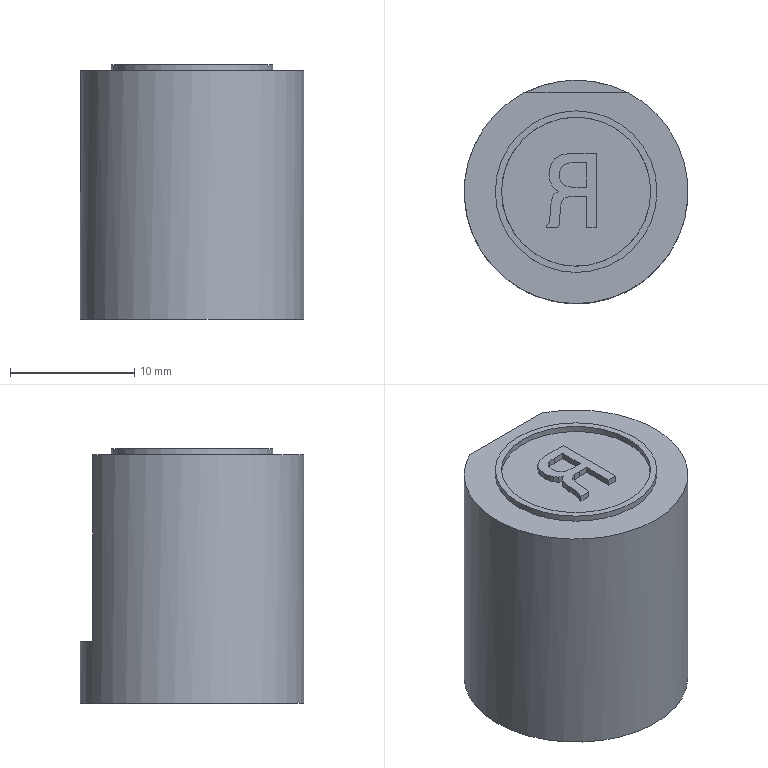Part | STEP file | lll_id4346_x_t | 1 solid | 50 faces | box 18 x 18 x 20.5 mm | volume 5022 mm3 | plane 47 | cylinder 3 | commonest cylinder face diameters 12 x1 13 x1 18 x1
STEP:
#1=CARTESIAN_POINT('',(396.,100.,0.));
#2=VERTEX_POINT('',#1);
#3=CARTESIAN_POINT('',(389.5,100.,0.));
#4=DIRECTION('',(0.,0.,-1.));
#5=DIRECTION('',(1.,0.,0.));
#6=AXIS2_PLACEMENT_3D('',#3,#4,#5);
#7=CIRCLE('',#6,6.5);
#8=EDGE_CURVE('',#2,#2,#7,.T.);
#9=ORIENTED_EDGE('',*,*,#8,.T.);
#10=EDGE_LOOP('',(#9));
#11=FACE_BOUND('',#10,.T.);
#12=CARTESIAN_POINT('',(393.623,108.,0.));
#13=VERTEX_POINT('',#12);
#14=CARTESIAN_POINT('',(385.377,108.,0.));
#15=VERTEX_POINT('',#14);
#16=CARTESIAN_POINT('',(389.5,108.,0.));
#17=DIRECTION('',(-1.,0.,0.));
#18=VECTOR('',#17,1.);
#19=LINE('',#16,#18);
#20=EDGE_CURVE('',#13,#15,#19,.T.);
#21=ORIENTED_EDGE('',*,*,#20,.T.);
#22=CARTESIAN_POINT('',(389.5,100.,0.));
#23=DIRECTION('',(0.,0.,-1.));
#24=DIRECTION('',(-1.,0.,0.));
#25=AXIS2_PLACEMENT_3D('',#22,#23,#24);
#26=CIRCLE('',#25,9.);
#27=EDGE_CURVE('',#13,#15,#26,.T.);
#28=ORIENTED_EDGE('',*,*,#27,.F.);
#29=EDGE_LOOP('',(#21,#28));
#30=FACE_BOUND('',#29,.T.);
#31=CARTESIAN_POINT('',(389.5,100.,0.));
#32=DIRECTION('',(0.,0.,1.));
#33=DIRECTION('',(1.,0.,0.));
#34=AXIS2_PLACEMENT_3D('',#31,#32,#33);
#35=PLANE('',#34);
#36=ADVANCED_FACE('',(#11,#30),#35,.T.);
#37=CARTESIAN_POINT('',(395.5,100.,0.));
#38=VERTEX_POINT('',#37);
#39=CARTESIAN_POINT('',(389.5,100.,0.));
#40=DIRECTION('',(0.,0.,1.));
#41=DIRECTION('',(1.,0.,0.));
#42=AXIS2_PLACEMENT_3D('',#39,#40,#41);
#43=CIRCLE('',#42,6.);
#44=EDGE_CURVE('',#38,#38,#43,.T.);
#45=ORIENTED_EDGE('',*,*,#44,.T.);
#46=EDGE_LOOP('',(#45));
#47=FACE_BOUND('',#46,.T.);
#48=CARTESIAN_POINT('',(388.133,97.386,0.));
#49=VERTEX_POINT('',#48);
#50=CARTESIAN_POINT('',(388.185,97.896,0.));
#51=VERTEX_POINT('',#50);
#52=CARTESIAN_POINT('',(388.133,97.386,0.));
#53=DIRECTION('',(0.1012,0.9949,0.));
#54=VECTOR('',#53,1.);
#55=LINE('',#52,#54);
#56=EDGE_CURVE('',#49,#51,#55,.T.);
#57=ORIENTED_EDGE('',*,*,#56,.F.);
#58=CARTESIAN_POINT('',(388.029,97.083,0.));
#59=VERTEX_POINT('',#58);
#60=CARTESIAN_POINT('',(388.029,97.083,0.));
#61=DIRECTION('',(-0.3242,-0.946,0.));
#62=VECTOR('',#61,1.);
#63=LINE('',#60,#62);
#64=EDGE_CURVE('',#49,#59,#63,.T.);
#65=ORIENTED_EDGE('',*,*,#64,.T.);
#66=CARTESIAN_POINT('',(387.121,97.083,0.));
#67=VERTEX_POINT('',#66);
#68=CARTESIAN_POINT('',(387.121,97.083,0.));
#69=DIRECTION('',(-1.,0.,0.));
#70=VECTOR('',#69,1.);
#71=LINE('',#68,#70);
#72=EDGE_CURVE('',#59,#67,#71,.T.);
#73=ORIENTED_EDGE('',*,*,#72,.T.);
#74=CARTESIAN_POINT('',(387.121,97.247,0.));
#75=VERTEX_POINT('',#74);
#76=CARTESIAN_POINT('',(387.121,97.247,0.));
#77=DIRECTION('',(0.,1.,0.));
#78=VECTOR('',#77,1.);
#79=LINE('',#76,#78);
#80=EDGE_CURVE('',#67,#75,#79,.T.);
#81=ORIENTED_EDGE('',*,*,#80,.T.);
#82=CARTESIAN_POINT('',(387.32,97.489,0.));
#83=VERTEX_POINT('',#82);
#84=CARTESIAN_POINT('',(387.32,97.489,0.));
#85=DIRECTION('',(0.6346,0.7728,0.));
#86=VECTOR('',#85,1.);
#87=LINE('',#84,#86);
#88=EDGE_CURVE('',#75,#83,#87,.T.);
#89=ORIENTED_EDGE('',*,*,#88,.T.);
#90=CARTESIAN_POINT('',(387.389,97.939,0.));
#91=VERTEX_POINT('',#90);
#92=CARTESIAN_POINT('',(387.389,97.939,0.));
#93=DIRECTION('',(0.1522,0.9884,0.));
#94=VECTOR('',#93,1.);
#95=LINE('',#92,#94);
#96=EDGE_CURVE('',#83,#91,#95,.T.);
#97=ORIENTED_EDGE('',*,*,#96,.T.);
#98=CARTESIAN_POINT('',(387.45,98.907,0.));
#99=VERTEX_POINT('',#98);
#100=CARTESIAN_POINT('',(387.45,98.907,0.));
#101=DIRECTION('',(-0.06234,-0.9981,0.));
#102=VECTOR('',#101,1.);
#103=LINE('',#100,#102);
#104=EDGE_CURVE('',#99,#91,#103,.T.);
#105=ORIENTED_EDGE('',*,*,#104,.F.);
#106=CARTESIAN_POINT('',(387.597,99.625,0.));
#107=VERTEX_POINT('',#106);
#108=CARTESIAN_POINT('',(387.597,99.625,0.));
#109=DIRECTION('',(-0.2007,-0.9797,0.));
#110=VECTOR('',#109,1.);
#111=LINE('',#108,#110);
#112=EDGE_CURVE('',#107,#99,#111,.T.);
#113=ORIENTED_EDGE('',*,*,#112,.F.);
#114=CARTESIAN_POINT('',(387.796,99.85,0.));
#115=VERTEX_POINT('',#114);
#116=CARTESIAN_POINT('',(387.796,99.85,0.));
#117=DIRECTION('',(0.6626,0.749,0.));
#118=VECTOR('',#117,1.);
#119=LINE('',#116,#118);
#120=EDGE_CURVE('',#107,#115,#119,.T.);
#121=ORIENTED_EDGE('',*,*,#120,.T.);
#122=CARTESIAN_POINT('',(388.107,100.014,0.));
#123=VERTEX_POINT('',#122);
#124=CARTESIAN_POINT('',(388.107,100.014,0.));
#125=DIRECTION('',(0.8844,0.4668,0.));
#126=VECTOR('',#125,1.);
#127=LINE('',#124,#126);
#128=EDGE_CURVE('',#115,#123,#127,.T.);
#129=ORIENTED_EDGE('',*,*,#128,.T.);
#130=CARTESIAN_POINT('',(387.761,100.23,0.));
#131=VERTEX_POINT('',#130);
#132=CARTESIAN_POINT('',(387.761,100.23,0.));
#133=DIRECTION('',(0.848,-0.53,0.));
#134=VECTOR('',#133,1.);
#135=LINE('',#132,#134);
#136=EDGE_CURVE('',#131,#123,#135,.T.);
#137=ORIENTED_EDGE('',*,*,#136,.F.);
#138=CARTESIAN_POINT('',(387.519,100.533,0.));
#139=VERTEX_POINT('',#138);
#140=CARTESIAN_POINT('',(387.519,100.533,0.));
#141=DIRECTION('',(-0.6248,0.7808,0.));
#142=VECTOR('',#141,1.);
#143=LINE('',#140,#142);
#144=EDGE_CURVE('',#131,#139,#143,.T.);
#145=ORIENTED_EDGE('',*,*,#144,.T.);
#146=CARTESIAN_POINT('',(387.363,100.913,0.));
#147=VERTEX_POINT('',#146);
#148=CARTESIAN_POINT('',(387.363,100.913,0.));
#149=DIRECTION('',(0.3785,-0.9256,0.));
#150=VECTOR('',#149,1.);
#151=LINE('',#148,#150);
#152=EDGE_CURVE('',#147,#139,#151,.T.);
#153=ORIENTED_EDGE('',*,*,#152,.F.);
#154=CARTESIAN_POINT('',(387.312,101.371,0.));
#155=VERTEX_POINT('',#154);
#156=CARTESIAN_POINT('',(387.312,101.371,0.));
#157=DIRECTION('',(-0.1125,0.9937,0.));
#158=VECTOR('',#157,1.);
#159=LINE('',#156,#158);
#160=EDGE_CURVE('',#147,#155,#159,.T.);
#161=ORIENTED_EDGE('',*,*,#160,.T.);
#162=CARTESIAN_POINT('',(387.433,102.098,0.));
#163=VERTEX_POINT('',#162);
#164=CARTESIAN_POINT('',(387.433,102.098,0.));
#165=DIRECTION('',(-0.1644,-0.9864,0.));
#166=VECTOR('',#165,1.);
#167=LINE('',#164,#166);
#168=EDGE_CURVE('',#163,#155,#167,.T.);
#169=ORIENTED_EDGE('',*,*,#168,.F.);
#170=CARTESIAN_POINT('',(387.778,102.642,0.));
#171=VERTEX_POINT('',#170);
#172=CARTESIAN_POINT('',(387.778,102.642,0.));
#173=DIRECTION('',(0.536,0.8442,0.));
#174=VECTOR('',#173,1.);
#175=LINE('',#172,#174);
#176=EDGE_CURVE('',#163,#171,#175,.T.);
#177=ORIENTED_EDGE('',*,*,#176,.T.);
#178=CARTESIAN_POINT('',(388.349,102.971,0.));
#179=VERTEX_POINT('',#178);
#180=CARTESIAN_POINT('',(388.349,102.971,0.));
#181=DIRECTION('',(0.8666,0.4989,0.));
#182=VECTOR('',#181,1.);
#183=LINE('',#180,#182);
#184=EDGE_CURVE('',#171,#179,#183,.T.);
#185=ORIENTED_EDGE('',*,*,#184,.T.);
#186=CARTESIAN_POINT('',(389.127,103.083,0.));
#187=VERTEX_POINT('',#186);
#188=CARTESIAN_POINT('',(389.127,103.083,0.));
#189=DIRECTION('',(0.9897,0.143,0.));
#190=VECTOR('',#189,1.);
#191=LINE('',#188,#190);
#192=EDGE_CURVE('',#179,#187,#191,.T.);
#193=ORIENTED_EDGE('',*,*,#192,.T.);
#194=CARTESIAN_POINT('',(391.133,103.083,0.));
#195=VERTEX_POINT('',#194);
#196=CARTESIAN_POINT('',(391.133,103.083,0.));
#197=DIRECTION('',(-1.,0.,0.));
#198=VECTOR('',#197,1.);
#199=LINE('',#196,#198);
#200=EDGE_CURVE('',#195,#187,#199,.T.);
#201=ORIENTED_EDGE('',*,*,#200,.F.);
#202=CARTESIAN_POINT('',(391.133,97.083,0.));
#203=VERTEX_POINT('',#202);
#204=CARTESIAN_POINT('',(391.133,97.083,0.));
#205=DIRECTION('',(0.,-1.,0.));
#206=VECTOR('',#205,1.);
#207=LINE('',#204,#206);
#208=EDGE_CURVE('',#195,#203,#207,.T.);
#209=ORIENTED_EDGE('',*,*,#208,.T.);
#210=CARTESIAN_POINT('',(390.329,97.083,0.));
#211=VERTEX_POINT('',#210);
#212=CARTESIAN_POINT('',(390.329,97.083,0.));
#213=DIRECTION('',(1.,0.,0.));
#214=VECTOR('',#213,1.);
#215=LINE('',#212,#214);
#216=EDGE_CURVE('',#211,#203,#215,.T.);
#217=ORIENTED_EDGE('',*,*,#216,.F.);
#218=CARTESIAN_POINT('',(390.329,99.616,0.));
#219=VERTEX_POINT('',#218);
#220=CARTESIAN_POINT('',(390.329,99.616,0.));
#221=DIRECTION('',(0.,-1.,0.));
#222=VECTOR('',#221,1.);
#223=LINE('',#220,#222);
#224=EDGE_CURVE('',#219,#211,#223,.T.);
#225=ORIENTED_EDGE('',*,*,#224,.F.);
#226=CARTESIAN_POINT('',(389.508,99.616,0.));
#227=VERTEX_POINT('',#226);
#228=CARTESIAN_POINT('',(389.508,99.616,0.));
#229=DIRECTION('',(-1.,0.,0.));
#230=VECTOR('',#229,1.);
#231=LINE('',#228,#230);
#232=EDGE_CURVE('',#219,#227,#231,.T.);
#233=ORIENTED_EDGE('',*,*,#232,.T.);
#234=CARTESIAN_POINT('',(388.902,99.59,0.));
#235=VERTEX_POINT('',#234);
#236=CARTESIAN_POINT('',(388.902,99.59,0.));
#237=DIRECTION('',(-0.9991,-0.04282,0.));
#238=VECTOR('',#237,1.);
#239=LINE('',#236,#238);
#240=EDGE_CURVE('',#227,#235,#239,.T.);
#241=ORIENTED_EDGE('',*,*,#240,.T.);
#242=CARTESIAN_POINT('',(388.522,99.469,0.));
#243=VERTEX_POINT('',#242);
#244=CARTESIAN_POINT('',(388.522,99.469,0.));
#245=DIRECTION('',(0.9529,0.3032,0.));
#246=VECTOR('',#245,1.);
#247=LINE('',#244,#246);
#248=EDGE_CURVE('',#243,#235,#247,.T.);
#249=ORIENTED_EDGE('',*,*,#248,.F.);
#250=CARTESIAN_POINT('',(388.314,99.184,0.));
#251=VERTEX_POINT('',#250);
#252=CARTESIAN_POINT('',(388.314,99.184,0.));
#253=DIRECTION('',(-0.5882,-0.8087,0.));
#254=VECTOR('',#253,1.);
#255=LINE('',#252,#254);
#256=EDGE_CURVE('',#243,#251,#255,.T.);
#257=ORIENTED_EDGE('',*,*,#256,.T.);
#258=CARTESIAN_POINT('',(388.228,98.674,0.));
#259=VERTEX_POINT('',#258);
#260=CARTESIAN_POINT('',(388.228,98.674,0.));
#261=DIRECTION('',(0.1671,0.9859,0.));
#262=VECTOR('',#261,1.);
#263=LINE('',#260,#262);
#264=EDGE_CURVE('',#259,#251,#263,.T.);
#265=ORIENTED_EDGE('',*,*,#264,.F.);
#266=CARTESIAN_POINT('',(388.185,97.896,0.));
#267=DIRECTION('',(-0.05553,-0.9985,0.));
#268=VECTOR('',#267,1.);
#269=LINE('',#266,#268);
#270=EDGE_CURVE('',#259,#51,#269,.T.);
#271=ORIENTED_EDGE('',*,*,#270,.T.);
#272=EDGE_LOOP('',(#57,#65,#73,#81,#89,#97,#105,#113,#121,#129,#137,#145,#153,#161,#169,#177,#185,#193,#201,#209,#217,#225,#233,#241,#249,#257,#265,#271));
#273=FACE_BOUND('',#272,.T.);
#274=CARTESIAN_POINT('',(389.5,100.,0.));
#275=DIRECTION('',(0.,0.,1.));
#276=DIRECTION('',(1.,0.,0.));
#277=AXIS2_PLACEMENT_3D('',#274,#275,#276);
#278=PLANE('',#277);
#279=ADVANCED_FACE('',(#47,#273),#278,.T.);
#280=ORIENTED_EDGE('',*,*,#8,.F.);
#281=EDGE_LOOP('',(#280));
#282=FACE_BOUND('',#281,.T.);
#283=CARTESIAN_POINT('',(383.,100.,0.5));
#284=VERTEX_POINT('',#283);
#285=CARTESIAN_POINT('',(389.5,100.,0.5));
#286=DIRECTION('',(0.,0.,1.));
#287=DIRECTION('',(-1.,0.,0.));
#288=AXIS2_PLACEMENT_3D('',#285,#286,#287);
#289=CIRCLE('',#288,6.5);
#290=EDGE_CURVE('',#284,#284,#289,.T.);
#291=ORIENTED_EDGE('',*,*,#290,.F.);
#292=EDGE_LOOP('',(#291));
#293=FACE_BOUND('',#292,.T.);
#294=CARTESIAN_POINT('',(389.5,100.,-2.));
#295=DIRECTION('',(0.,0.,1.));
#296=DIRECTION('',(1.,0.,0.));
#297=AXIS2_PLACEMENT_3D('',#294,#295,#296);
#298=CYLINDRICAL_SURFACE('',#297,6.5);
#299=ADVANCED_FACE('',(#282,#293),#298,.T.);
#300=ORIENTED_EDGE('',*,*,#290,.T.);
#301=EDGE_LOOP('',(#300));
#302=FACE_BOUND('',#301,.T.);
#303=CARTESIAN_POINT('',(383.5,100.,0.5));
#304=VERTEX_POINT('',#303);
#305=CARTESIAN_POINT('',(389.5,100.,0.5));
#306=DIRECTION('',(0.,0.,-1.));
#307=DIRECTION('',(-1.,0.,0.));
#308=AXIS2_PLACEMENT_3D('',#305,#306,#307);
#309=CIRCLE('',#308,6.);
#310=EDGE_CURVE('',#304,#304,#309,.T.);
#311=ORIENTED_EDGE('',*,*,#310,.T.);
#312=EDGE_LOOP('',(#311));
#313=FACE_BOUND('',#312,.T.);
#314=CARTESIAN_POINT('',(389.5,100.,0.5));
#315=DIRECTION('',(0.,0.,1.));
#316=DIRECTION('',(1.,0.,0.));
#317=AXIS2_PLACEMENT_3D('',#314,#315,#316);
#318=PLANE('',#317);
#319=ADVANCED_FACE('',(#302,#313),#318,.T.);
#320=ORIENTED_EDGE('',*,*,#44,.F.);
#321=EDGE_LOOP('',(#320));
#322=FACE_BOUND('',#321,.T.);
#323=ORIENTED_EDGE('',*,*,#310,.F.);
#324=EDGE_LOOP('',(#323));
#325=FACE_BOUND('',#324,.T.);
#326=CARTESIAN_POINT('',(389.5,100.,-2.));
#327=DIRECTION('',(0.,0.,1.));
#328=DIRECTION('',(1.,0.,0.));
#329=AXIS2_PLACEMENT_3D('',#326,#327,#328);
#330=CYLINDRICAL_SURFACE('',#329,6.);
#331=ADVANCED_FACE('',(#322,#325),#330,.F.);
#332=CARTESIAN_POINT('',(388.219,101.83,0.));
#333=VERTEX_POINT('',#332);
#334=CARTESIAN_POINT('',(388.219,101.83,0.5));
#335=VERTEX_POINT('',#334);
#336=CARTESIAN_POINT('',(388.219,101.83,-2.));
#337=DIRECTION('',(0.,0.,1.));
#338=VECTOR('',#337,1.);
#339=LINE('',#336,#338);
#340=EDGE_CURVE('',#333,#335,#339,.T.);
#341=ORIENTED_EDGE('',*,*,#340,.F.);
#342=CARTESIAN_POINT('',(388.453,102.132,0.));
#343=VERTEX_POINT('',#342);
#344=CARTESIAN_POINT('',(388.453,102.132,0.));
#345=DIRECTION('',(0.6108,0.7918,0.));
#346=VECTOR('',#345,1.);
#347=LINE('',#344,#346);
#348=EDGE_CURVE('',#333,#343,#347,.T.);
#349=ORIENTED_EDGE('',*,*,#348,.T.);
#350=CARTESIAN_POINT('',(388.453,102.132,0.5));
#351=VERTEX_POINT('',#350);
#352=CARTESIAN_POINT('',(388.453,102.132,-2.));
#353=DIRECTION('',(0.,0.,1.));
#354=VECTOR('',#353,1.);
#355=LINE('',#352,#354);
#356=EDGE_CURVE('',#343,#351,#355,.T.);
#357=ORIENTED_EDGE('',*,*,#356,.T.);
#358=CARTESIAN_POINT('',(388.453,102.132,0.5));
#359=DIRECTION('',(-0.6108,-0.7918,0.));
#360=VECTOR('',#359,1.);
#361=LINE('',#358,#360);
#362=EDGE_CURVE('',#351,#335,#361,.T.);
#363=ORIENTED_EDGE('',*,*,#362,.T.);
#364=EDGE_LOOP('',(#341,#349,#357,#363));
#365=FACE_OUTER_BOUND('',#364,.T.);
#366=CARTESIAN_POINT('',(388.453,102.132,-2.));
#367=DIRECTION('',(-0.7918,0.6108,0.));
#368=DIRECTION('',(0.6108,0.7918,0.));
#369=AXIS2_PLACEMENT_3D('',#366,#367,#368);
#370=PLANE('',#369);
#371=ADVANCED_FACE('',(#365),#370,.F.);
#372=ORIENTED_EDGE('',*,*,#356,.F.);
#373=CARTESIAN_POINT('',(388.825,102.296,0.));
#374=VERTEX_POINT('',#373);
#375=CARTESIAN_POINT('',(388.825,102.296,0.));
#376=DIRECTION('',(-0.9147,-0.4042,0.));
#377=VECTOR('',#376,1.);
#378=LINE('',#375,#377);
#379=EDGE_CURVE('',#374,#343,#378,.T.);
#380=ORIENTED_EDGE('',*,*,#379,.F.);
#381=CARTESIAN_POINT('',(388.825,102.296,0.5));
#382=VERTEX_POINT('',#381);
#383=CARTESIAN_POINT('',(388.825,102.296,-2.));
#384=DIRECTION('',(0.,0.,1.));
#385=VECTOR('',#384,1.);
#386=LINE('',#383,#385);
#387=EDGE_CURVE('',#374,#382,#386,.T.);
#388=ORIENTED_EDGE('',*,*,#387,.T.);
#389=CARTESIAN_POINT('',(388.825,102.296,0.5));
#390=DIRECTION('',(-0.9147,-0.4042,0.));
#391=VECTOR('',#390,1.);
#392=LINE('',#389,#391);
#393=EDGE_CURVE('',#382,#351,#392,.T.);
#394=ORIENTED_EDGE('',*,*,#393,.T.);
#395=EDGE_LOOP('',(#372,#380,#388,#394));
#396=FACE_OUTER_BOUND('',#395,.T.);
#397=CARTESIAN_POINT('',(388.825,102.296,-2.));
#398=DIRECTION('',(-0.4042,0.9147,0.));
#399=DIRECTION('',(0.9147,0.4042,0.));
#400=AXIS2_PLACEMENT_3D('',#397,#398,#399);
#401=PLANE('',#400);
#402=ADVANCED_FACE('',(#396),#401,.F.);
#403=ORIENTED_EDGE('',*,*,#387,.F.);
#404=CARTESIAN_POINT('',(389.352,102.348,0.));
#405=VERTEX_POINT('',#404);
#406=CARTESIAN_POINT('',(389.352,102.348,0.));
#407=DIRECTION('',(0.9952,0.0979,0.));
#408=VECTOR('',#407,1.);
#409=LINE('',#406,#408);
#410=EDGE_CURVE('',#374,#405,#409,.T.);
#411=ORIENTED_EDGE('',*,*,#410,.T.);
#412=CARTESIAN_POINT('',(389.352,102.348,0.5));
#413=VERTEX_POINT('',#412);
#414=CARTESIAN_POINT('',(389.352,102.348,-2.));
#415=DIRECTION('',(0.,0.,1.));
#416=VECTOR('',#415,1.);
#417=LINE('',#414,#416);
#418=EDGE_CURVE('',#405,#413,#417,.T.);
#419=ORIENTED_EDGE('',*,*,#418,.T.);
#420=CARTESIAN_POINT('',(389.352,102.348,0.5));
#421=DIRECTION('',(-0.9952,-0.0979,0.));
#422=VECTOR('',#421,1.);
#423=LINE('',#420,#422);
#424=EDGE_CURVE('',#413,#382,#423,.T.);
#425=ORIENTED_EDGE('',*,*,#424,.T.);
#426=EDGE_LOOP('',(#403,#411,#419,#425));
#427=FACE_OUTER_BOUND('',#426,.T.);
#428=CARTESIAN_POINT('',(389.352,102.348,-2.));
#429=DIRECTION('',(-0.0979,0.9952,0.));
#430=DIRECTION('',(0.9952,0.0979,0.));
#431=AXIS2_PLACEMENT_3D('',#428,#429,#430);
#432=PLANE('',#431);
#433=ADVANCED_FACE('',(#427),#432,.F.);
#434=ORIENTED_EDGE('',*,*,#418,.F.);
#435=CARTESIAN_POINT('',(390.329,102.348,0.));
#436=VERTEX_POINT('',#435);
#437=CARTESIAN_POINT('',(390.329,102.348,0.));
#438=DIRECTION('',(1.,0.,0.));
#439=VECTOR('',#438,1.);
#440=LINE('',#437,#439);
#441=EDGE_CURVE('',#405,#436,#440,.T.);
#442=ORIENTED_EDGE('',*,*,#441,.T.);
#443=CARTESIAN_POINT('',(390.329,102.348,0.5));
#444=VERTEX_POINT('',#443);
#445=CARTESIAN_POINT('',(390.329,102.348,-2.));
#446=DIRECTION('',(0.,0.,1.));
#447=VECTOR('',#446,1.);
#448=LINE('',#445,#447);
#449=EDGE_CURVE('',#436,#444,#448,.T.);
#450=ORIENTED_EDGE('',*,*,#449,.T.);
#451=CARTESIAN_POINT('',(390.329,102.348,0.5));
#452=DIRECTION('',(-1.,0.,0.));
#453=VECTOR('',#452,1.);
#454=LINE('',#451,#453);
#455=EDGE_CURVE('',#444,#413,#454,.T.);
#456=ORIENTED_EDGE('',*,*,#455,.T.);
#457=EDGE_LOOP('',(#434,#442,#450,#456));
#458=FACE_OUTER_BOUND('',#457,.T.);
#459=CARTESIAN_POINT('',(390.329,102.348,-2.));
#460=DIRECTION('',(0.,1.,0.));
#461=DIRECTION('',(0.,0.,1.));
#462=AXIS2_PLACEMENT_3D('',#459,#460,#461);
#463=PLANE('',#462);
#464=ADVANCED_FACE('',(#458),#463,.F.);
#465=ORIENTED_EDGE('',*,*,#449,.F.);
#466=CARTESIAN_POINT('',(390.329,100.351,0.));
#467=VERTEX_POINT('',#466);
#468=CARTESIAN_POINT('',(390.329,100.351,0.));
#469=DIRECTION('',(0.,1.,0.));
#470=VECTOR('',#469,1.);
#471=LINE('',#468,#470);
#472=EDGE_CURVE('',#467,#436,#471,.T.);
#473=ORIENTED_EDGE('',*,*,#472,.F.);
#474=CARTESIAN_POINT('',(390.329,100.351,0.5));
#475=VERTEX_POINT('',#474);
#476=CARTESIAN_POINT('',(390.329,100.351,-2.));
#477=DIRECTION('',(0.,0.,1.));
#478=VECTOR('',#477,1.);
#479=LINE('',#476,#478);
#480=EDGE_CURVE('',#467,#475,#479,.T.);
#481=ORIENTED_EDGE('',*,*,#480,.T.);
#482=CARTESIAN_POINT('',(390.329,100.351,0.5));
#483=DIRECTION('',(0.,1.,0.));
#484=VECTOR('',#483,1.);
#485=LINE('',#482,#484);
#486=EDGE_CURVE('',#475,#444,#485,.T.);
#487=ORIENTED_EDGE('',*,*,#486,.T.);
#488=EDGE_LOOP('',(#465,#473,#481,#487));
#489=FACE_OUTER_BOUND('',#488,.T.);
#490=CARTESIAN_POINT('',(390.329,100.351,-2.));
#491=DIRECTION('',(1.,0.,0.));
#492=DIRECTION('',(0.,0.,-1.));
#493=AXIS2_PLACEMENT_3D('',#490,#491,#492);
#494=PLANE('',#493);
#495=ADVANCED_FACE('',(#489),#494,.F.);
#496=ORIENTED_EDGE('',*,*,#480,.F.);
#497=CARTESIAN_POINT('',(389.404,100.351,0.));
#498=VERTEX_POINT('',#497);
#499=CARTESIAN_POINT('',(389.404,100.351,0.));
#500=DIRECTION('',(-1.,0.,0.));
#501=VECTOR('',#500,1.);
#502=LINE('',#499,#501);
#503=EDGE_CURVE('',#467,#498,#502,.T.);
#504=ORIENTED_EDGE('',*,*,#503,.T.);
#505=CARTESIAN_POINT('',(389.404,100.351,0.5));
#506=VERTEX_POINT('',#505);
#507=CARTESIAN_POINT('',(389.404,100.351,-2.));
#508=DIRECTION('',(0.,0.,1.));
#509=VECTOR('',#508,1.);
#510=LINE('',#507,#509);
#511=EDGE_CURVE('',#498,#506,#510,.T.);
#512=ORIENTED_EDGE('',*,*,#511,.T.);
#513=CARTESIAN_POINT('',(389.404,100.351,0.5));
#514=DIRECTION('',(1.,0.,0.));
#515=VECTOR('',#514,1.);
#516=LINE('',#513,#515);
#517=EDGE_CURVE('',#506,#475,#516,.T.);
#518=ORIENTED_EDGE('',*,*,#517,.T.);
#519=EDGE_LOOP('',(#496,#504,#512,#518));
#520=FACE_OUTER_BOUND('',#519,.T.);
#521=CARTESIAN_POINT('',(389.404,100.351,-2.));
#522=DIRECTION('',(0.,-1.,0.));
#523=DIRECTION('',(0.,0.,-1.));
#524=AXIS2_PLACEMENT_3D('',#521,#522,#523);
#525=PLANE('',#524);
#526=ADVANCED_FACE('',(#520),#525,.F.);
#527=ORIENTED_EDGE('',*,*,#511,.F.);
#528=CARTESIAN_POINT('',(388.859,100.394,0.));
#529=VERTEX_POINT('',#528);
#530=CARTESIAN_POINT('',(388.859,100.394,0.));
#531=DIRECTION('',(0.9969,-0.07914,0.));
#532=VECTOR('',#531,1.);
#533=LINE('',#530,#532);
#534=EDGE_CURVE('',#529,#498,#533,.T.);
#535=ORIENTED_EDGE('',*,*,#534,.F.);
#536=CARTESIAN_POINT('',(388.859,100.394,0.5));
#537=VERTEX_POINT('',#536);
#538=CARTESIAN_POINT('',(388.859,100.394,-2.));
#539=DIRECTION('',(0.,0.,1.));
#540=VECTOR('',#539,1.);
#541=LINE('',#538,#540);
#542=EDGE_CURVE('',#529,#537,#541,.T.);
#543=ORIENTED_EDGE('',*,*,#542,.T.);
#544=CARTESIAN_POINT('',(388.859,100.394,0.5));
#545=DIRECTION('',(0.9969,-0.07914,0.));
#546=VECTOR('',#545,1.);
#547=LINE('',#544,#546);
#548=EDGE_CURVE('',#537,#506,#547,.T.);
#549=ORIENTED_EDGE('',*,*,#548,.T.);
#550=EDGE_LOOP('',(#527,#535,#543,#549));
#551=FACE_OUTER_BOUND('',#550,.T.);
#552=CARTESIAN_POINT('',(388.859,100.394,-2.));
#553=DIRECTION('',(-0.07914,-0.9969,0.));
#554=DIRECTION('',(-0.9969,0.07914,0.));
#555=AXIS2_PLACEMENT_3D('',#552,#553,#554);
#556=PLANE('',#555);
#557=ADVANCED_FACE('',(#551),#556,.F.);
#558=ORIENTED_EDGE('',*,*,#542,.F.);
#559=CARTESIAN_POINT('',(388.461,100.55,0.));
#560=VERTEX_POINT('',#559);
#561=CARTESIAN_POINT('',(388.461,100.55,0.));
#562=DIRECTION('',(-0.9313,0.3644,0.));
#563=VECTOR('',#562,1.);
#564=LINE('',#561,#563);
#565=EDGE_CURVE('',#529,#560,#564,.T.);
#566=ORIENTED_EDGE('',*,*,#565,.T.);
#567=CARTESIAN_POINT('',(388.461,100.55,0.5));
#568=VERTEX_POINT('',#567);
#569=CARTESIAN_POINT('',(388.461,100.55,-2.));
#570=DIRECTION('',(0.,0.,1.));
#571=VECTOR('',#570,1.);
#572=LINE('',#569,#571);
#573=EDGE_CURVE('',#560,#568,#572,.T.);
#574=ORIENTED_EDGE('',*,*,#573,.T.);
#575=CARTESIAN_POINT('',(388.461,100.55,0.5));
#576=DIRECTION('',(0.9313,-0.3644,0.));
#577=VECTOR('',#576,1.);
#578=LINE('',#575,#577);
#579=EDGE_CURVE('',#568,#537,#578,.T.);
#580=ORIENTED_EDGE('',*,*,#579,.T.);
#581=EDGE_LOOP('',(#558,#566,#574,#580));
#582=FACE_OUTER_BOUND('',#581,.T.);
#583=CARTESIAN_POINT('',(388.461,100.55,-2.));
#584=DIRECTION('',(-0.3644,-0.9313,0.));
#585=DIRECTION('',(-0.9313,0.3644,0.));
#586=AXIS2_PLACEMENT_3D('',#583,#584,#585);
#587=PLANE('',#586);
#588=ADVANCED_FACE('',(#582),#587,.F.);
#589=ORIENTED_EDGE('',*,*,#573,.F.);
#590=CARTESIAN_POINT('',(388.228,100.853,0.));
#591=VERTEX_POINT('',#590);
#592=CARTESIAN_POINT('',(388.228,100.853,0.));
#593=DIRECTION('',(-0.6108,0.7918,0.));
#594=VECTOR('',#593,1.);
#595=LINE('',#592,#594);
#596=EDGE_CURVE('',#560,#591,#595,.T.);
#597=ORIENTED_EDGE('',*,*,#596,.T.);
#598=CARTESIAN_POINT('',(388.228,100.853,0.5));
#599=VERTEX_POINT('',#598);
#600=CARTESIAN_POINT('',(388.228,100.853,-2.));
#601=DIRECTION('',(0.,0.,1.));
#602=VECTOR('',#601,1.);
#603=LINE('',#600,#602);
#604=EDGE_CURVE('',#591,#599,#603,.T.);
#605=ORIENTED_EDGE('',*,*,#604,.T.);
#606=CARTESIAN_POINT('',(388.228,100.853,0.5));
#607=DIRECTION('',(0.6108,-0.7918,0.));
#608=VECTOR('',#607,1.);
#609=LINE('',#606,#608);
#610=EDGE_CURVE('',#599,#568,#609,.T.);
#611=ORIENTED_EDGE('',*,*,#610,.T.);
#612=EDGE_LOOP('',(#589,#597,#605,#611));
#613=FACE_OUTER_BOUND('',#612,.T.);
#614=CARTESIAN_POINT('',(388.228,100.853,-2.));
#615=DIRECTION('',(-0.7918,-0.6108,0.));
#616=DIRECTION('',(-0.6108,0.7918,0.));
#617=AXIS2_PLACEMENT_3D('',#614,#615,#616);
#618=PLANE('',#617);
#619=ADVANCED_FACE('',(#613),#618,.F.);
#620=ORIENTED_EDGE('',*,*,#604,.F.);
#621=CARTESIAN_POINT('',(388.142,101.354,0.));
#622=VERTEX_POINT('',#621);
#623=CARTESIAN_POINT('',(388.142,101.354,0.));
#624=DIRECTION('',(-0.17,0.9855,0.));
#625=VECTOR('',#624,1.);
#626=LINE('',#623,#625);
#627=EDGE_CURVE('',#591,#622,#626,.T.);
#628=ORIENTED_EDGE('',*,*,#627,.T.);
#629=CARTESIAN_POINT('',(388.142,101.354,0.5));
#630=VERTEX_POINT('',#629);
#631=CARTESIAN_POINT('',(388.142,101.354,-2.));
#632=DIRECTION('',(0.,0.,1.));
#633=VECTOR('',#632,1.);
#634=LINE('',#631,#633);
#635=EDGE_CURVE('',#622,#630,#634,.T.);
#636=ORIENTED_EDGE('',*,*,#635,.T.);
#637=CARTESIAN_POINT('',(388.142,101.354,0.5));
#638=DIRECTION('',(0.17,-0.9855,0.));
#639=VECTOR('',#638,1.);
#640=LINE('',#637,#639);
#641=EDGE_CURVE('',#630,#599,#640,.T.);
#642=ORIENTED_EDGE('',*,*,#641,.T.);
#643=EDGE_LOOP('',(#620,#628,#636,#642));
#644=FACE_OUTER_BOUND('',#643,.T.);
#645=CARTESIAN_POINT('',(388.142,101.354,-2.));
#646=DIRECTION('',(-0.9855,-0.17,0.));
#647=DIRECTION('',(-0.17,0.9855,0.));
#648=AXIS2_PLACEMENT_3D('',#645,#646,#647);
#649=PLANE('',#648);
#650=ADVANCED_FACE('',(#644),#649,.F.);
#651=ORIENTED_EDGE('',*,*,#635,.F.);
#652=CARTESIAN_POINT('',(388.219,101.83,0.));
#653=DIRECTION('',(0.1615,0.9869,0.));
#654=VECTOR('',#653,1.);
#655=LINE('',#652,#654);
#656=EDGE_CURVE('',#622,#333,#655,.T.);
#657=ORIENTED_EDGE('',*,*,#656,.T.);
#658=ORIENTED_EDGE('',*,*,#340,.T.);
#659=CARTESIAN_POINT('',(388.219,101.83,0.5));
#660=DIRECTION('',(-0.1615,-0.9869,0.));
#661=VECTOR('',#660,1.);
#662=LINE('',#659,#661);
#663=EDGE_CURVE('',#335,#630,#662,.T.);
#664=ORIENTED_EDGE('',*,*,#663,.T.);
#665=EDGE_LOOP('',(#651,#657,#658,#664));
#666=FACE_OUTER_BOUND('',#665,.T.);
#667=CARTESIAN_POINT('',(388.219,101.83,-2.));
#668=DIRECTION('',(-0.9869,0.1615,0.));
#669=DIRECTION('',(0.1615,0.9869,0.));
#670=AXIS2_PLACEMENT_3D('',#667,#668,#669);
#671=PLANE('',#670);
#672=ADVANCED_FACE('',(#666),#671,.F.);
#673=CARTESIAN_POINT('',(387.121,97.247,0.5));
#674=VERTEX_POINT('',#673);
#675=CARTESIAN_POINT('',(387.121,97.083,0.5));
#676=VERTEX_POINT('',#675);
#677=CARTESIAN_POINT('',(387.121,97.247,0.5));
#678=DIRECTION('',(0.,-1.,0.));
#679=VECTOR('',#678,1.);
#680=LINE('',#677,#679);
#681=EDGE_CURVE('',#674,#676,#680,.T.);
#682=ORIENTED_EDGE('',*,*,#681,.T.);
#683=CARTESIAN_POINT('',(388.029,97.083,0.5));
#684=VERTEX_POINT('',#683);
#685=CARTESIAN_POINT('',(387.121,97.083,0.5));
#686=DIRECTION('',(1.,0.,0.));
#687=VECTOR('',#686,1.);
#688=LINE('',#685,#687);
#689=EDGE_CURVE('',#676,#684,#688,.T.);
#690=ORIENTED_EDGE('',*,*,#689,.T.);
#691=CARTESIAN_POINT('',(388.133,97.386,0.5));
#692=VERTEX_POINT('',#691);
#693=CARTESIAN_POINT('',(388.029,97.083,0.5));
#694=DIRECTION('',(0.3242,0.946,0.));
#695=VECTOR('',#694,1.);
#696=LINE('',#693,#695);
#697=EDGE_CURVE('',#684,#692,#696,.T.);
#698=ORIENTED_EDGE('',*,*,#697,.T.);
#699=CARTESIAN_POINT('',(388.185,97.896,0.5));
#700=VERTEX_POINT('',#699);
#701=CARTESIAN_POINT('',(388.133,97.386,0.5));
#702=DIRECTION('',(0.1012,0.9949,0.));
#703=VECTOR('',#702,1.);
#704=LINE('',#701,#703);
#705=EDGE_CURVE('',#692,#700,#704,.T.);
#706=ORIENTED_EDGE('',*,*,#705,.T.);
#707=CARTESIAN_POINT('',(388.228,98.674,0.5));
#708=VERTEX_POINT('',#707);
#709=CARTESIAN_POINT('',(388.185,97.896,0.5));
#710=DIRECTION('',(0.05553,0.9985,0.));
#711=VECTOR('',#710,1.);
#712=LINE('',#709,#711);
#713=EDGE_CURVE('',#700,#708,#712,.T.);
#714=ORIENTED_EDGE('',*,*,#713,.T.);
#715=CARTESIAN_POINT('',(388.314,99.184,0.5));
#716=VERTEX_POINT('',#715);
#717=CARTESIAN_POINT('',(388.228,98.674,0.5));
#718=DIRECTION('',(0.1671,0.9859,0.));
#719=VECTOR('',#718,1.);
#720=LINE('',#717,#719);
#721=EDGE_CURVE('',#708,#716,#720,.T.);
#722=ORIENTED_EDGE('',*,*,#721,.T.);
#723=CARTESIAN_POINT('',(388.522,99.469,0.5));
#724=VERTEX_POINT('',#723);
#725=CARTESIAN_POINT('',(388.314,99.184,0.5));
#726=DIRECTION('',(0.5882,0.8087,0.));
#727=VECTOR('',#726,1.);
#728=LINE('',#725,#727);
#729=EDGE_CURVE('',#716,#724,#728,.T.);
#730=ORIENTED_EDGE('',*,*,#729,.T.);
#731=CARTESIAN_POINT('',(388.902,99.59,0.5));
#732=VERTEX_POINT('',#731);
#733=CARTESIAN_POINT('',(388.522,99.469,0.5));
#734=DIRECTION('',(0.9529,0.3032,0.));
#735=VECTOR('',#734,1.);
#736=LINE('',#733,#735);
#737=EDGE_CURVE('',#724,#732,#736,.T.);
#738=ORIENTED_EDGE('',*,*,#737,.T.);
#739=CARTESIAN_POINT('',(389.508,99.616,0.5));
#740=VERTEX_POINT('',#739);
#741=CARTESIAN_POINT('',(388.902,99.59,0.5));
#742=DIRECTION('',(0.9991,0.04282,0.));
#743=VECTOR('',#742,1.);
#744=LINE('',#741,#743);
#745=EDGE_CURVE('',#732,#740,#744,.T.);
#746=ORIENTED_EDGE('',*,*,#745,.T.);
#747=CARTESIAN_POINT('',(390.329,99.616,0.5));
#748=VERTEX_POINT('',#747);
#749=CARTESIAN_POINT('',(389.508,99.616,0.5));
#750=DIRECTION('',(1.,0.,0.));
#751=VECTOR('',#750,1.);
#752=LINE('',#749,#751);
#753=EDGE_CURVE('',#740,#748,#752,.T.);
#754=ORIENTED_EDGE('',*,*,#753,.T.);
#755=CARTESIAN_POINT('',(390.329,97.083,0.5));
#756=VERTEX_POINT('',#755);
#757=CARTESIAN_POINT('',(390.329,99.616,0.5));
#758=DIRECTION('',(0.,-1.,0.));
#759=VECTOR('',#758,1.);
#760=LINE('',#757,#759);
#761=EDGE_CURVE('',#748,#756,#760,.T.);
#762=ORIENTED_EDGE('',*,*,#761,.T.);
#763=CARTESIAN_POINT('',(391.133,97.083,0.5));
#764=VERTEX_POINT('',#763);
#765=CARTESIAN_POINT('',(390.329,97.083,0.5));
#766=DIRECTION('',(1.,0.,0.));
#767=VECTOR('',#766,1.);
#768=LINE('',#765,#767);
#769=EDGE_CURVE('',#756,#764,#768,.T.);
#770=ORIENTED_EDGE('',*,*,#769,.T.);
#771=CARTESIAN_POINT('',(391.133,103.083,0.5));
#772=VERTEX_POINT('',#771);
#773=CARTESIAN_POINT('',(391.133,97.083,0.5));
#774=DIRECTION('',(0.,1.,0.));
#775=VECTOR('',#774,1.);
#776=LINE('',#773,#775);
#777=EDGE_CURVE('',#764,#772,#776,.T.);
#778=ORIENTED_EDGE('',*,*,#777,.T.);
#779=CARTESIAN_POINT('',(389.127,103.083,0.5));
#780=VERTEX_POINT('',#779);
#781=CARTESIAN_POINT('',(391.133,103.083,0.5));
#782=DIRECTION('',(-1.,0.,0.));
#783=VECTOR('',#782,1.);
#784=LINE('',#781,#783);
#785=EDGE_CURVE('',#772,#780,#784,.T.);
#786=ORIENTED_EDGE('',*,*,#785,.T.);
#787=CARTESIAN_POINT('',(388.349,102.971,0.5));
#788=VERTEX_POINT('',#787);
#789=CARTESIAN_POINT('',(389.127,103.083,0.5));
#790=DIRECTION('',(-0.9897,-0.143,0.));
#791=VECTOR('',#790,1.);
#792=LINE('',#789,#791);
#793=EDGE_CURVE('',#780,#788,#792,.T.);
#794=ORIENTED_EDGE('',*,*,#793,.T.);
#795=CARTESIAN_POINT('',(387.778,102.642,0.5));
#796=VERTEX_POINT('',#795);
#797=CARTESIAN_POINT('',(388.349,102.971,0.5));
#798=DIRECTION('',(-0.8666,-0.4989,0.));
#799=VECTOR('',#798,1.);
#800=LINE('',#797,#799);
#801=EDGE_CURVE('',#788,#796,#800,.T.);
#802=ORIENTED_EDGE('',*,*,#801,.T.);
#803=CARTESIAN_POINT('',(387.433,102.098,0.5));
#804=VERTEX_POINT('',#803);
#805=CARTESIAN_POINT('',(387.778,102.642,0.5));
#806=DIRECTION('',(-0.536,-0.8442,0.));
#807=VECTOR('',#806,1.);
#808=LINE('',#805,#807);
#809=EDGE_CURVE('',#796,#804,#808,.T.);
#810=ORIENTED_EDGE('',*,*,#809,.T.);
#811=CARTESIAN_POINT('',(387.312,101.371,0.5));
#812=VERTEX_POINT('',#811);
#813=CARTESIAN_POINT('',(387.433,102.098,0.5));
#814=DIRECTION('',(-0.1644,-0.9864,0.));
#815=VECTOR('',#814,1.);
#816=LINE('',#813,#815);
#817=EDGE_CURVE('',#804,#812,#816,.T.);
#818=ORIENTED_EDGE('',*,*,#817,.T.);
#819=CARTESIAN_POINT('',(387.363,100.913,0.5));
#820=VERTEX_POINT('',#819);
#821=CARTESIAN_POINT('',(387.312,101.371,0.5));
#822=DIRECTION('',(0.1125,-0.9937,0.));
#823=VECTOR('',#822,1.);
#824=LINE('',#821,#823);
#825=EDGE_CURVE('',#812,#820,#824,.T.);
#826=ORIENTED_EDGE('',*,*,#825,.T.);
#827=CARTESIAN_POINT('',(387.519,100.533,0.5));
#828=VERTEX_POINT('',#827);
#829=CARTESIAN_POINT('',(387.363,100.913,0.5));
#830=DIRECTION('',(0.3785,-0.9256,0.));
#831=VECTOR('',#830,1.);
#832=LINE('',#829,#831);
#833=EDGE_CURVE('',#820,#828,#832,.T.);
#834=ORIENTED_EDGE('',*,*,#833,.T.);
#835=CARTESIAN_POINT('',(387.761,100.23,0.5));
#836=VERTEX_POINT('',#835);
#837=CARTESIAN_POINT('',(387.519,100.533,0.5));
#838=DIRECTION('',(0.6248,-0.7808,0.));
#839=VECTOR('',#838,1.);
#840=LINE('',#837,#839);
#841=EDGE_CURVE('',#828,#836,#840,.T.);
#842=ORIENTED_EDGE('',*,*,#841,.T.);
#843=CARTESIAN_POINT('',(388.107,100.014,0.5));
#844=VERTEX_POINT('',#843);
#845=CARTESIAN_POINT('',(387.761,100.23,0.5));
#846=DIRECTION('',(0.848,-0.53,0.));
#847=VECTOR('',#846,1.);
#848=LINE('',#845,#847);
#849=EDGE_CURVE('',#836,#844,#848,.T.);
#850=ORIENTED_EDGE('',*,*,#849,.T.);
#851=CARTESIAN_POINT('',(387.796,99.85,0.5));
#852=VERTEX_POINT('',#851);
#853=CARTESIAN_POINT('',(388.107,100.014,0.5));
#854=DIRECTION('',(-0.8844,-0.4668,0.));
#855=VECTOR('',#854,1.);
#856=LINE('',#853,#855);
#857=EDGE_CURVE('',#844,#852,#856,.T.);
#858=ORIENTED_EDGE('',*,*,#857,.T.);
#859=CARTESIAN_POINT('',(387.597,99.625,0.5));
#860=VERTEX_POINT('',#859);
#861=CARTESIAN_POINT('',(387.796,99.85,0.5));
#862=DIRECTION('',(-0.6626,-0.749,0.));
#863=VECTOR('',#862,1.);
#864=LINE('',#861,#863);
#865=EDGE_CURVE('',#852,#860,#864,.T.);
#866=ORIENTED_EDGE('',*,*,#865,.T.);
#867=CARTESIAN_POINT('',(387.45,98.907,0.5));
#868=VERTEX_POINT('',#867);
#869=CARTESIAN_POINT('',(387.597,99.625,0.5));
#870=DIRECTION('',(-0.2007,-0.9797,0.));
#871=VECTOR('',#870,1.);
#872=LINE('',#869,#871);
#873=EDGE_CURVE('',#860,#868,#872,.T.);
#874=ORIENTED_EDGE('',*,*,#873,.T.);
#875=CARTESIAN_POINT('',(387.389,97.939,0.5));
#876=VERTEX_POINT('',#875);
#877=CARTESIAN_POINT('',(387.45,98.907,0.5));
#878=DIRECTION('',(-0.06234,-0.9981,0.));
#879=VECTOR('',#878,1.);
#880=LINE('',#877,#879);
#881=EDGE_CURVE('',#868,#876,#880,.T.);
#882=ORIENTED_EDGE('',*,*,#881,.T.);
#883=CARTESIAN_POINT('',(387.32,97.489,0.5));
#884=VERTEX_POINT('',#883);
#885=CARTESIAN_POINT('',(387.389,97.939,0.5));
#886=DIRECTION('',(-0.1522,-0.9884,0.));
#887=VECTOR('',#886,1.);
#888=LINE('',#885,#887);
#889=EDGE_CURVE('',#876,#884,#888,.T.);
#890=ORIENTED_EDGE('',*,*,#889,.T.);
#891=CARTESIAN_POINT('',(387.32,97.489,0.5));
#892=DIRECTION('',(-0.6346,-0.7728,0.));
#893=VECTOR('',#892,1.);
#894=LINE('',#891,#893);
#895=EDGE_CURVE('',#884,#674,#894,.T.);
#896=ORIENTED_EDGE('',*,*,#895,.T.);
#897=EDGE_LOOP('',(#682,#690,#698,#706,#714,#722,#730,#738,#746,#754,#762,#770,#778,#786,#794,#802,#810,#818,#826,#834,#842,#850,#858,#866,#874,#882,#890,#896));
#898=FACE_BOUND('',#897,.T.);
#899=ORIENTED_EDGE('',*,*,#362,.F.);
#900=ORIENTED_EDGE('',*,*,#393,.F.);
#901=ORIENTED_EDGE('',*,*,#424,.F.);
#902=ORIENTED_EDGE('',*,*,#455,.F.);
#903=ORIENTED_EDGE('',*,*,#486,.F.);
#904=ORIENTED_EDGE('',*,*,#517,.F.);
#905=ORIENTED_EDGE('',*,*,#548,.F.);
#906=ORIENTED_EDGE('',*,*,#579,.F.);
#907=ORIENTED_EDGE('',*,*,#610,.F.);
#908=ORIENTED_EDGE('',*,*,#641,.F.);
#909=ORIENTED_EDGE('',*,*,#663,.F.);
#910=EDGE_LOOP('',(#899,#900,#901,#902,#903,#904,#905,#906,#907,#908,#909));
#911=FACE_BOUND('',#910,.T.);
#912=CARTESIAN_POINT('',(-2493.249,1.,0.5));
#913=DIRECTION('',(0.,0.,1.));
#914=DIRECTION('',(1.,0.,0.));
#915=AXIS2_PLACEMENT_3D('',#912,#913,#914);
#916=PLANE('',#915);
#917=ADVANCED_FACE('',(#898,#911),#916,.T.);
#918=ORIENTED_EDGE('',*,*,#56,.T.);
#919=CARTESIAN_POINT('',(388.185,97.896,-2.));
#920=DIRECTION('',(0.,0.,1.));
#921=VECTOR('',#920,1.);
#922=LINE('',#919,#921);
#923=EDGE_CURVE('',#51,#700,#922,.T.);
#924=ORIENTED_EDGE('',*,*,#923,.T.);
#925=ORIENTED_EDGE('',*,*,#705,.F.);
#926=CARTESIAN_POINT('',(388.133,97.386,-2.));
#927=DIRECTION('',(0.,0.,1.));
#928=VECTOR('',#927,1.);
#929=LINE('',#926,#928);
#930=EDGE_CURVE('',#49,#692,#929,.T.);
#931=ORIENTED_EDGE('',*,*,#930,.F.);
#932=EDGE_LOOP('',(#918,#924,#925,#931));
#933=FACE_OUTER_BOUND('',#932,.T.);
#934=CARTESIAN_POINT('',(388.133,97.386,-2.));
#935=DIRECTION('',(0.9949,-0.1012,0.));
#936=DIRECTION('',(-0.1012,-0.9949,0.));
#937=AXIS2_PLACEMENT_3D('',#934,#935,#936);
#938=PLANE('',#937);
#939=ADVANCED_FACE('',(#933),#938,.T.);
#940=ORIENTED_EDGE('',*,*,#270,.F.);
#941=CARTESIAN_POINT('',(388.228,98.674,-2.));
#942=DIRECTION('',(0.,0.,1.));
#943=VECTOR('',#942,1.);
#944=LINE('',#941,#943);
#945=EDGE_CURVE('',#259,#708,#944,.T.);
#946=ORIENTED_EDGE('',*,*,#945,.T.);
#947=ORIENTED_EDGE('',*,*,#713,.F.);
#948=ORIENTED_EDGE('',*,*,#923,.F.);
#949=EDGE_LOOP('',(#940,#946,#947,#948));
#950=FACE_OUTER_BOUND('',#949,.T.);
#951=CARTESIAN_POINT('',(388.185,97.896,-2.));
#952=DIRECTION('',(0.9985,-0.05553,0.));
#953=DIRECTION('',(-0.05553,-0.9985,0.));
#954=AXIS2_PLACEMENT_3D('',#951,#952,#953);
#955=PLANE('',#954);
#956=ADVANCED_FACE('',(#950),#955,.T.);
#957=ORIENTED_EDGE('',*,*,#264,.T.);
#958=CARTESIAN_POINT('',(388.314,99.184,-2.));
#959=DIRECTION('',(0.,0.,1.));
#960=VECTOR('',#959,1.);
#961=LINE('',#958,#960);
#962=EDGE_CURVE('',#251,#716,#961,.T.);
#963=ORIENTED_EDGE('',*,*,#962,.T.);
#964=ORIENTED_EDGE('',*,*,#721,.F.);
#965=ORIENTED_EDGE('',*,*,#945,.F.);
#966=EDGE_LOOP('',(#957,#963,#964,#965));
#967=FACE_OUTER_BOUND('',#966,.T.);
#968=CARTESIAN_POINT('',(388.228,98.674,-2.));
#969=DIRECTION('',(0.9859,-0.1671,0.));
#970=DIRECTION('',(-0.1671,-0.9859,0.));
#971=AXIS2_PLACEMENT_3D('',#968,#969,#970);
#972=PLANE('',#971);
#973=ADVANCED_FACE('',(#967),#972,.T.);
#974=ORIENTED_EDGE('',*,*,#256,.F.);
#975=CARTESIAN_POINT('',(388.522,99.469,-2.));
#976=DIRECTION('',(0.,0.,1.));
#977=VECTOR('',#976,1.);
#978=LINE('',#975,#977);
#979=EDGE_CURVE('',#243,#724,#978,.T.);
#980=ORIENTED_EDGE('',*,*,#979,.T.);
#981=ORIENTED_EDGE('',*,*,#729,.F.);
#982=ORIENTED_EDGE('',*,*,#962,.F.);
#983=EDGE_LOOP('',(#974,#980,#981,#982));
#984=FACE_OUTER_BOUND('',#983,.T.);
#985=CARTESIAN_POINT('',(388.314,99.184,-2.));
#986=DIRECTION('',(0.8087,-0.5882,0.));
#987=DIRECTION('',(-0.5882,-0.8087,0.));
#988=AXIS2_PLACEMENT_3D('',#985,#986,#987);
#989=PLANE('',#988);
#990=ADVANCED_FACE('',(#984),#989,.T.);
#991=ORIENTED_EDGE('',*,*,#248,.T.);
#992=CARTESIAN_POINT('',(388.902,99.59,-2.));
#993=DIRECTION('',(0.,0.,1.));
#994=VECTOR('',#993,1.);
#995=LINE('',#992,#994);
#996=EDGE_CURVE('',#235,#732,#995,.T.);
#997=ORIENTED_EDGE('',*,*,#996,.T.);
#998=ORIENTED_EDGE('',*,*,#737,.F.);
#999=ORIENTED_EDGE('',*,*,#979,.F.);
#1000=EDGE_LOOP('',(#991,#997,#998,#999));
#1001=FACE_OUTER_BOUND('',#1000,.T.);
#1002=CARTESIAN_POINT('',(388.522,99.469,-2.));
#1003=DIRECTION('',(0.3032,-0.9529,0.));
#1004=DIRECTION('',(-0.9529,-0.3032,0.));
#1005=AXIS2_PLACEMENT_3D('',#1002,#1003,#1004);
#1006=PLANE('',#1005);
#1007=ADVANCED_FACE('',(#1001),#1006,.T.);
#1008=ORIENTED_EDGE('',*,*,#240,.F.);
#1009=CARTESIAN_POINT('',(389.508,99.616,-2.));
#1010=DIRECTION('',(0.,0.,1.));
#1011=VECTOR('',#1010,1.);
#1012=LINE('',#1009,#1011);
#1013=EDGE_CURVE('',#227,#740,#1012,.T.);
#1014=ORIENTED_EDGE('',*,*,#1013,.T.);
#1015=ORIENTED_EDGE('',*,*,#745,.F.);
#1016=ORIENTED_EDGE('',*,*,#996,.F.);
#1017=EDGE_LOOP('',(#1008,#1014,#1015,#1016));
#1018=FACE_OUTER_BOUND('',#1017,.T.);
#1019=CARTESIAN_POINT('',(388.902,99.59,-2.));
#1020=DIRECTION('',(0.04282,-0.9991,0.));
#1021=DIRECTION('',(-0.9991,-0.04282,0.));
#1022=AXIS2_PLACEMENT_3D('',#1019,#1020,#1021);
#1023=PLANE('',#1022);
#1024=ADVANCED_FACE('',(#1018),#1023,.T.);
#1025=ORIENTED_EDGE('',*,*,#232,.F.);
#1026=CARTESIAN_POINT('',(390.329,99.616,-2.));
#1027=DIRECTION('',(0.,0.,1.));
#1028=VECTOR('',#1027,1.);
#1029=LINE('',#1026,#1028);
#1030=EDGE_CURVE('',#219,#748,#1029,.T.);
#1031=ORIENTED_EDGE('',*,*,#1030,.T.);
#1032=ORIENTED_EDGE('',*,*,#753,.F.);
#1033=ORIENTED_EDGE('',*,*,#1013,.F.);
#1034=EDGE_LOOP('',(#1025,#1031,#1032,#1033));
#1035=FACE_OUTER_BOUND('',#1034,.T.);
#1036=CARTESIAN_POINT('',(389.508,99.616,-2.));
#1037=DIRECTION('',(0.,-1.,0.));
#1038=DIRECTION('',(0.,0.,-1.));
#1039=AXIS2_PLACEMENT_3D('',#1036,#1037,#1038);
#1040=PLANE('',#1039);
#1041=ADVANCED_FACE('',(#1035),#1040,.T.);
#1042=ORIENTED_EDGE('',*,*,#224,.T.);
#1043=CARTESIAN_POINT('',(390.329,97.083,-2.));
#1044=DIRECTION('',(0.,0.,1.));
#1045=VECTOR('',#1044,1.);
#1046=LINE('',#1043,#1045);
#1047=EDGE_CURVE('',#211,#756,#1046,.T.);
#1048=ORIENTED_EDGE('',*,*,#1047,.T.);
#1049=ORIENTED_EDGE('',*,*,#761,.F.);
#1050=ORIENTED_EDGE('',*,*,#1030,.F.);
#1051=EDGE_LOOP('',(#1042,#1048,#1049,#1050));
#1052=FACE_OUTER_BOUND('',#1051,.T.);
#1053=CARTESIAN_POINT('',(390.329,99.616,-2.));
#1054=DIRECTION('',(-1.,0.,0.));
#1055=DIRECTION('',(0.,0.,1.));
#1056=AXIS2_PLACEMENT_3D('',#1053,#1054,#1055);
#1057=PLANE('',#1056);
#1058=ADVANCED_FACE('',(#1052),#1057,.T.);
#1059=ORIENTED_EDGE('',*,*,#216,.T.);
#1060=CARTESIAN_POINT('',(391.133,97.083,-2.));
#1061=DIRECTION('',(0.,0.,1.));
#1062=VECTOR('',#1061,1.);
#1063=LINE('',#1060,#1062);
#1064=EDGE_CURVE('',#203,#764,#1063,.T.);
#1065=ORIENTED_EDGE('',*,*,#1064,.T.);
#1066=ORIENTED_EDGE('',*,*,#769,.F.);
#1067=ORIENTED_EDGE('',*,*,#1047,.F.);
#1068=EDGE_LOOP('',(#1059,#1065,#1066,#1067));
#1069=FACE_OUTER_BOUND('',#1068,.T.);
#1070=CARTESIAN_POINT('',(390.329,97.083,-2.));
#1071=DIRECTION('',(0.,-1.,0.));
#1072=DIRECTION('',(0.,0.,-1.));
#1073=AXIS2_PLACEMENT_3D('',#1070,#1071,#1072);
#1074=PLANE('',#1073);
#1075=ADVANCED_FACE('',(#1069),#1074,.T.);
#1076=ORIENTED_EDGE('',*,*,#208,.F.);
#1077=CARTESIAN_POINT('',(391.133,103.083,-2.));
#1078=DIRECTION('',(0.,0.,1.));
#1079=VECTOR('',#1078,1.);
#1080=LINE('',#1077,#1079);
#1081=EDGE_CURVE('',#195,#772,#1080,.T.);
#1082=ORIENTED_EDGE('',*,*,#1081,.T.);
#1083=ORIENTED_EDGE('',*,*,#777,.F.);
#1084=ORIENTED_EDGE('',*,*,#1064,.F.);
#1085=EDGE_LOOP('',(#1076,#1082,#1083,#1084));
#1086=FACE_OUTER_BOUND('',#1085,.T.);
#1087=CARTESIAN_POINT('',(391.133,97.083,-2.));
#1088=DIRECTION('',(1.,0.,0.));
#1089=DIRECTION('',(0.,0.,-1.));
#1090=AXIS2_PLACEMENT_3D('',#1087,#1088,#1089);
#1091=PLANE('',#1090);
#1092=ADVANCED_FACE('',(#1086),#1091,.T.);
#1093=ORIENTED_EDGE('',*,*,#200,.T.);
#1094=CARTESIAN_POINT('',(389.127,103.083,-2.));
#1095=DIRECTION('',(0.,0.,1.));
#1096=VECTOR('',#1095,1.);
#1097=LINE('',#1094,#1096);
#1098=EDGE_CURVE('',#187,#780,#1097,.T.);
#1099=ORIENTED_EDGE('',*,*,#1098,.T.);
#1100=ORIENTED_EDGE('',*,*,#785,.F.);
#1101=ORIENTED_EDGE('',*,*,#1081,.F.);
#1102=EDGE_LOOP('',(#1093,#1099,#1100,#1101));
#1103=FACE_OUTER_BOUND('',#1102,.T.);
#1104=CARTESIAN_POINT('',(391.133,103.083,-2.));
#1105=DIRECTION('',(0.,1.,0.));
#1106=DIRECTION('',(0.,0.,1.));
#1107=AXIS2_PLACEMENT_3D('',#1104,#1105,#1106);
#1108=PLANE('',#1107);
#1109=ADVANCED_FACE('',(#1103),#1108,.T.);
#1110=ORIENTED_EDGE('',*,*,#192,.F.);
#1111=CARTESIAN_POINT('',(388.349,102.971,-2.));
#1112=DIRECTION('',(0.,0.,1.));
#1113=VECTOR('',#1112,1.);
#1114=LINE('',#1111,#1113);
#1115=EDGE_CURVE('',#179,#788,#1114,.T.);
#1116=ORIENTED_EDGE('',*,*,#1115,.T.);
#1117=ORIENTED_EDGE('',*,*,#793,.F.);
#1118=ORIENTED_EDGE('',*,*,#1098,.F.);
#1119=EDGE_LOOP('',(#1110,#1116,#1117,#1118));
#1120=FACE_OUTER_BOUND('',#1119,.T.);
#1121=CARTESIAN_POINT('',(389.127,103.083,-2.));
#1122=DIRECTION('',(-0.143,0.9897,0.));
#1123=DIRECTION('',(0.9897,0.143,0.));
#1124=AXIS2_PLACEMENT_3D('',#1121,#1122,#1123);
#1125=PLANE('',#1124);
#1126=ADVANCED_FACE('',(#1120),#1125,.T.);
#1127=ORIENTED_EDGE('',*,*,#184,.F.);
#1128=CARTESIAN_POINT('',(387.778,102.642,-2.));
#1129=DIRECTION('',(0.,0.,1.));
#1130=VECTOR('',#1129,1.);
#1131=LINE('',#1128,#1130);
#1132=EDGE_CURVE('',#171,#796,#1131,.T.);
#1133=ORIENTED_EDGE('',*,*,#1132,.T.);
#1134=ORIENTED_EDGE('',*,*,#801,.F.);
#1135=ORIENTED_EDGE('',*,*,#1115,.F.);
#1136=EDGE_LOOP('',(#1127,#1133,#1134,#1135));
#1137=FACE_OUTER_BOUND('',#1136,.T.);
#1138=CARTESIAN_POINT('',(388.349,102.971,-2.));
#1139=DIRECTION('',(-0.4989,0.8666,0.));
#1140=DIRECTION('',(0.8666,0.4989,0.));
#1141=AXIS2_PLACEMENT_3D('',#1138,#1139,#1140);
#1142=PLANE('',#1141);
#1143=ADVANCED_FACE('',(#1137),#1142,.T.);
#1144=ORIENTED_EDGE('',*,*,#176,.F.);
#1145=CARTESIAN_POINT('',(387.433,102.098,-2.));
#1146=DIRECTION('',(0.,0.,1.));
#1147=VECTOR('',#1146,1.);
#1148=LINE('',#1145,#1147);
#1149=EDGE_CURVE('',#163,#804,#1148,.T.);
#1150=ORIENTED_EDGE('',*,*,#1149,.T.);
#1151=ORIENTED_EDGE('',*,*,#809,.F.);
#1152=ORIENTED_EDGE('',*,*,#1132,.F.);
#1153=EDGE_LOOP('',(#1144,#1150,#1151,#1152));
#1154=FACE_OUTER_BOUND('',#1153,.T.);
#1155=CARTESIAN_POINT('',(387.778,102.642,-2.));
#1156=DIRECTION('',(-0.8442,0.536,0.));
#1157=DIRECTION('',(0.536,0.8442,0.));
#1158=AXIS2_PLACEMENT_3D('',#1155,#1156,#1157);
#1159=PLANE('',#1158);
#1160=ADVANCED_FACE('',(#1154),#1159,.T.);
#1161=ORIENTED_EDGE('',*,*,#168,.T.);
#1162=CARTESIAN_POINT('',(387.312,101.371,-2.));
#1163=DIRECTION('',(0.,0.,1.));
#1164=VECTOR('',#1163,1.);
#1165=LINE('',#1162,#1164);
#1166=EDGE_CURVE('',#155,#812,#1165,.T.);
#1167=ORIENTED_EDGE('',*,*,#1166,.T.);
#1168=ORIENTED_EDGE('',*,*,#817,.F.);
#1169=ORIENTED_EDGE('',*,*,#1149,.F.);
#1170=EDGE_LOOP('',(#1161,#1167,#1168,#1169));
#1171=FACE_OUTER_BOUND('',#1170,.T.);
#1172=CARTESIAN_POINT('',(387.433,102.098,-2.));
#1173=DIRECTION('',(-0.9864,0.1644,0.));
#1174=DIRECTION('',(0.1644,0.9864,0.));
#1175=AXIS2_PLACEMENT_3D('',#1172,#1173,#1174);
#1176=PLANE('',#1175);
#1177=ADVANCED_FACE('',(#1171),#1176,.T.);
#1178=ORIENTED_EDGE('',*,*,#160,.F.);
#1179=CARTESIAN_POINT('',(387.363,100.913,-2.));
#1180=DIRECTION('',(0.,0.,1.));
#1181=VECTOR('',#1180,1.);
#1182=LINE('',#1179,#1181);
#1183=EDGE_CURVE('',#147,#820,#1182,.T.);
#1184=ORIENTED_EDGE('',*,*,#1183,.T.);
#1185=ORIENTED_EDGE('',*,*,#825,.F.);
#1186=ORIENTED_EDGE('',*,*,#1166,.F.);
#1187=EDGE_LOOP('',(#1178,#1184,#1185,#1186));
#1188=FACE_OUTER_BOUND('',#1187,.T.);
#1189=CARTESIAN_POINT('',(387.312,101.371,-2.));
#1190=DIRECTION('',(-0.9937,-0.1125,0.));
#1191=DIRECTION('',(-0.1125,0.9937,0.));
#1192=AXIS2_PLACEMENT_3D('',#1189,#1190,#1191);
#1193=PLANE('',#1192);
#1194=ADVANCED_FACE('',(#1188),#1193,.T.);
#1195=ORIENTED_EDGE('',*,*,#152,.T.);
#1196=CARTESIAN_POINT('',(387.519,100.533,-2.));
#1197=DIRECTION('',(0.,0.,1.));
#1198=VECTOR('',#1197,1.);
#1199=LINE('',#1196,#1198);
#1200=EDGE_CURVE('',#139,#828,#1199,.T.);
#1201=ORIENTED_EDGE('',*,*,#1200,.T.);
#1202=ORIENTED_EDGE('',*,*,#833,.F.);
#1203=ORIENTED_EDGE('',*,*,#1183,.F.);
#1204=EDGE_LOOP('',(#1195,#1201,#1202,#1203));
#1205=FACE_OUTER_BOUND('',#1204,.T.);
#1206=CARTESIAN_POINT('',(387.363,100.913,-2.));
#1207=DIRECTION('',(-0.9256,-0.3785,0.));
#1208=DIRECTION('',(-0.3785,0.9256,0.));
#1209=AXIS2_PLACEMENT_3D('',#1206,#1207,#1208);
#1210=PLANE('',#1209);
#1211=ADVANCED_FACE('',(#1205),#1210,.T.);
#1212=ORIENTED_EDGE('',*,*,#144,.F.);
#1213=CARTESIAN_POINT('',(387.761,100.23,-2.));
#1214=DIRECTION('',(0.,0.,1.));
#1215=VECTOR('',#1214,1.);
#1216=LINE('',#1213,#1215);
#1217=EDGE_CURVE('',#131,#836,#1216,.T.);
#1218=ORIENTED_EDGE('',*,*,#1217,.T.);
#1219=ORIENTED_EDGE('',*,*,#841,.F.);
#1220=ORIENTED_EDGE('',*,*,#1200,.F.);
#1221=EDGE_LOOP('',(#1212,#1218,#1219,#1220));
#1222=FACE_OUTER_BOUND('',#1221,.T.);
#1223=CARTESIAN_POINT('',(387.519,100.533,-2.));
#1224=DIRECTION('',(-0.7808,-0.6248,0.));
#1225=DIRECTION('',(-0.6248,0.7808,0.));
#1226=AXIS2_PLACEMENT_3D('',#1223,#1224,#1225);
#1227=PLANE('',#1226);
#1228=ADVANCED_FACE('',(#1222),#1227,.T.);
#1229=ORIENTED_EDGE('',*,*,#136,.T.);
#1230=CARTESIAN_POINT('',(388.107,100.014,-2.));
#1231=DIRECTION('',(0.,0.,1.));
#1232=VECTOR('',#1231,1.);
#1233=LINE('',#1230,#1232);
#1234=EDGE_CURVE('',#123,#844,#1233,.T.);
#1235=ORIENTED_EDGE('',*,*,#1234,.T.);
#1236=ORIENTED_EDGE('',*,*,#849,.F.);
#1237=ORIENTED_EDGE('',*,*,#1217,.F.);
#1238=EDGE_LOOP('',(#1229,#1235,#1236,#1237));
#1239=FACE_OUTER_BOUND('',#1238,.T.);
#1240=CARTESIAN_POINT('',(387.761,100.23,-2.));
#1241=DIRECTION('',(-0.53,-0.848,0.));
#1242=DIRECTION('',(-0.848,0.53,0.));
#1243=AXIS2_PLACEMENT_3D('',#1240,#1241,#1242);
#1244=PLANE('',#1243);
#1245=ADVANCED_FACE('',(#1239),#1244,.T.);
#1246=ORIENTED_EDGE('',*,*,#128,.F.);
#1247=CARTESIAN_POINT('',(387.796,99.85,-2.));
#1248=DIRECTION('',(0.,0.,1.));
#1249=VECTOR('',#1248,1.);
#1250=LINE('',#1247,#1249);
#1251=EDGE_CURVE('',#115,#852,#1250,.T.);
#1252=ORIENTED_EDGE('',*,*,#1251,.T.);
#1253=ORIENTED_EDGE('',*,*,#857,.F.);
#1254=ORIENTED_EDGE('',*,*,#1234,.F.);
#1255=EDGE_LOOP('',(#1246,#1252,#1253,#1254));
#1256=FACE_OUTER_BOUND('',#1255,.T.);
#1257=CARTESIAN_POINT('',(388.107,100.014,-2.));
#1258=DIRECTION('',(-0.4668,0.8844,0.));
#1259=DIRECTION('',(0.8844,0.4668,0.));
#1260=AXIS2_PLACEMENT_3D('',#1257,#1258,#1259);
#1261=PLANE('',#1260);
#1262=ADVANCED_FACE('',(#1256),#1261,.T.);
#1263=ORIENTED_EDGE('',*,*,#120,.F.);
#1264=CARTESIAN_POINT('',(387.597,99.625,-2.));
#1265=DIRECTION('',(0.,0.,1.));
#1266=VECTOR('',#1265,1.);
#1267=LINE('',#1264,#1266);
#1268=EDGE_CURVE('',#107,#860,#1267,.T.);
#1269=ORIENTED_EDGE('',*,*,#1268,.T.);
#1270=ORIENTED_EDGE('',*,*,#865,.F.);
#1271=ORIENTED_EDGE('',*,*,#1251,.F.);
#1272=EDGE_LOOP('',(#1263,#1269,#1270,#1271));
#1273=FACE_OUTER_BOUND('',#1272,.T.);
#1274=CARTESIAN_POINT('',(387.796,99.85,-2.));
#1275=DIRECTION('',(-0.749,0.6626,0.));
#1276=DIRECTION('',(0.6626,0.749,0.));
#1277=AXIS2_PLACEMENT_3D('',#1274,#1275,#1276);
#1278=PLANE('',#1277);
#1279=ADVANCED_FACE('',(#1273),#1278,.T.);
#1280=ORIENTED_EDGE('',*,*,#112,.T.);
#1281=CARTESIAN_POINT('',(387.45,98.907,-2.));
#1282=DIRECTION('',(0.,0.,1.));
#1283=VECTOR('',#1282,1.);
#1284=LINE('',#1281,#1283);
#1285=EDGE_CURVE('',#99,#868,#1284,.T.);
#1286=ORIENTED_EDGE('',*,*,#1285,.T.);
#1287=ORIENTED_EDGE('',*,*,#873,.F.);
#1288=ORIENTED_EDGE('',*,*,#1268,.F.);
#1289=EDGE_LOOP('',(#1280,#1286,#1287,#1288));
#1290=FACE_OUTER_BOUND('',#1289,.T.);
#1291=CARTESIAN_POINT('',(387.597,99.625,-2.));
#1292=DIRECTION('',(-0.9797,0.2007,0.));
#1293=DIRECTION('',(0.2007,0.9797,0.));
#1294=AXIS2_PLACEMENT_3D('',#1291,#1292,#1293);
#1295=PLANE('',#1294);
#1296=ADVANCED_FACE('',(#1290),#1295,.T.);
#1297=ORIENTED_EDGE('',*,*,#104,.T.);
#1298=CARTESIAN_POINT('',(387.389,97.939,-2.));
#1299=DIRECTION('',(0.,0.,1.));
#1300=VECTOR('',#1299,1.);
#1301=LINE('',#1298,#1300);
#1302=EDGE_CURVE('',#91,#876,#1301,.T.);
#1303=ORIENTED_EDGE('',*,*,#1302,.T.);
#1304=ORIENTED_EDGE('',*,*,#881,.F.);
#1305=ORIENTED_EDGE('',*,*,#1285,.F.);
#1306=EDGE_LOOP('',(#1297,#1303,#1304,#1305));
#1307=FACE_OUTER_BOUND('',#1306,.T.);
#1308=CARTESIAN_POINT('',(387.45,98.907,-2.));
#1309=DIRECTION('',(-0.9981,0.06234,0.));
#1310=DIRECTION('',(0.06234,0.9981,0.));
#1311=AXIS2_PLACEMENT_3D('',#1308,#1309,#1310);
#1312=PLANE('',#1311);
#1313=ADVANCED_FACE('',(#1307),#1312,.T.);
#1314=ORIENTED_EDGE('',*,*,#96,.F.);
#1315=CARTESIAN_POINT('',(387.32,97.489,-2.));
#1316=DIRECTION('',(0.,0.,1.));
#1317=VECTOR('',#1316,1.);
#1318=LINE('',#1315,#1317);
#1319=EDGE_CURVE('',#83,#884,#1318,.T.);
#1320=ORIENTED_EDGE('',*,*,#1319,.T.);
#1321=ORIENTED_EDGE('',*,*,#889,.F.);
#1322=ORIENTED_EDGE('',*,*,#1302,.F.);
#1323=EDGE_LOOP('',(#1314,#1320,#1321,#1322));
#1324=FACE_OUTER_BOUND('',#1323,.T.);
#1325=CARTESIAN_POINT('',(387.389,97.939,-2.));
#1326=DIRECTION('',(-0.9884,0.1522,0.));
#1327=DIRECTION('',(0.1522,0.9884,0.));
#1328=AXIS2_PLACEMENT_3D('',#1325,#1326,#1327);
#1329=PLANE('',#1328);
#1330=ADVANCED_FACE('',(#1324),#1329,.T.);
#1331=ORIENTED_EDGE('',*,*,#88,.F.);
#1332=CARTESIAN_POINT('',(387.121,97.247,-2.));
#1333=DIRECTION('',(0.,0.,1.));
#1334=VECTOR('',#1333,1.);
#1335=LINE('',#1332,#1334);
#1336=EDGE_CURVE('',#75,#674,#1335,.T.);
#1337=ORIENTED_EDGE('',*,*,#1336,.T.);
#1338=ORIENTED_EDGE('',*,*,#895,.F.);
#1339=ORIENTED_EDGE('',*,*,#1319,.F.);
#1340=EDGE_LOOP('',(#1331,#1337,#1338,#1339));
#1341=FACE_OUTER_BOUND('',#1340,.T.);
#1342=CARTESIAN_POINT('',(387.32,97.489,-2.));
#1343=DIRECTION('',(-0.7728,0.6346,0.));
#1344=DIRECTION('',(0.6346,0.7728,0.));
#1345=AXIS2_PLACEMENT_3D('',#1342,#1343,#1344);
#1346=PLANE('',#1345);
#1347=ADVANCED_FACE('',(#1341),#1346,.T.);
#1348=ORIENTED_EDGE('',*,*,#80,.F.);
#1349=CARTESIAN_POINT('',(387.121,97.083,-2.));
#1350=DIRECTION('',(0.,0.,1.));
#1351=VECTOR('',#1350,1.);
#1352=LINE('',#1349,#1351);
#1353=EDGE_CURVE('',#67,#676,#1352,.T.);
#1354=ORIENTED_EDGE('',*,*,#1353,.T.);
#1355=ORIENTED_EDGE('',*,*,#681,.F.);
#1356=ORIENTED_EDGE('',*,*,#1336,.F.);
#1357=EDGE_LOOP('',(#1348,#1354,#1355,#1356));
#1358=FACE_OUTER_BOUND('',#1357,.T.);
#1359=CARTESIAN_POINT('',(387.121,97.247,-2.));
#1360=DIRECTION('',(-1.,0.,0.));
#1361=DIRECTION('',(0.,0.,1.));
#1362=AXIS2_PLACEMENT_3D('',#1359,#1360,#1361);
#1363=PLANE('',#1362);
#1364=ADVANCED_FACE('',(#1358),#1363,.T.);
#1365=ORIENTED_EDGE('',*,*,#72,.F.);
#1366=CARTESIAN_POINT('',(388.029,97.083,-2.));
#1367=DIRECTION('',(0.,0.,1.));
#1368=VECTOR('',#1367,1.);
#1369=LINE('',#1366,#1368);
#1370=EDGE_CURVE('',#59,#684,#1369,.T.);
#1371=ORIENTED_EDGE('',*,*,#1370,.T.);
#1372=ORIENTED_EDGE('',*,*,#689,.F.);
#1373=ORIENTED_EDGE('',*,*,#1353,.F.);
#1374=EDGE_LOOP('',(#1365,#1371,#1372,#1373));
#1375=FACE_OUTER_BOUND('',#1374,.T.);
#1376=CARTESIAN_POINT('',(387.121,97.083,-2.));
#1377=DIRECTION('',(0.,-1.,0.));
#1378=DIRECTION('',(0.,0.,-1.));
#1379=AXIS2_PLACEMENT_3D('',#1376,#1377,#1378);
#1380=PLANE('',#1379);
#1381=ADVANCED_FACE('',(#1375),#1380,.T.);
#1382=ORIENTED_EDGE('',*,*,#64,.F.);
#1383=ORIENTED_EDGE('',*,*,#930,.T.);
#1384=ORIENTED_EDGE('',*,*,#697,.F.);
#1385=ORIENTED_EDGE('',*,*,#1370,.F.);
#1386=EDGE_LOOP('',(#1382,#1383,#1384,#1385));
#1387=FACE_OUTER_BOUND('',#1386,.T.);
#1388=CARTESIAN_POINT('',(388.029,97.083,-2.));
#1389=DIRECTION('',(0.946,-0.3242,0.));
#1390=DIRECTION('',(-0.3242,-0.946,0.));
#1391=AXIS2_PLACEMENT_3D('',#1388,#1389,#1390);
#1392=PLANE('',#1391);
#1393=ADVANCED_FACE('',(#1387),#1392,.T.);
#1394=ORIENTED_EDGE('',*,*,#627,.F.);
#1395=ORIENTED_EDGE('',*,*,#596,.F.);
#1396=ORIENTED_EDGE('',*,*,#565,.F.);
#1397=ORIENTED_EDGE('',*,*,#534,.T.);
#1398=ORIENTED_EDGE('',*,*,#503,.F.);
#1399=ORIENTED_EDGE('',*,*,#472,.T.);
#1400=ORIENTED_EDGE('',*,*,#441,.F.);
#1401=ORIENTED_EDGE('',*,*,#410,.F.);
#1402=ORIENTED_EDGE('',*,*,#379,.T.);
#1403=ORIENTED_EDGE('',*,*,#348,.F.);
#1404=ORIENTED_EDGE('',*,*,#656,.F.);
#1405=EDGE_LOOP('',(#1394,#1395,#1396,#1397,#1398,#1399,#1400,#1401,#1402,#1403,#1404));
#1406=FACE_OUTER_BOUND('',#1405,.T.);
#1407=CARTESIAN_POINT('',(389.5,100.,0.));
#1408=DIRECTION('',(0.,0.,1.));
#1409=DIRECTION('',(1.,0.,0.));
#1410=AXIS2_PLACEMENT_3D('',#1407,#1408,#1409);
#1411=PLANE('',#1410);
#1412=ADVANCED_FACE('',(#1406),#1411,.T.);
#1413=CARTESIAN_POINT('',(380.5,100.,-20.));
#1414=VERTEX_POINT('',#1413);
#1415=CARTESIAN_POINT('',(389.5,100.,-20.));
#1416=DIRECTION('',(0.,0.,-1.));
#1417=DIRECTION('',(-1.,0.,0.));
#1418=AXIS2_PLACEMENT_3D('',#1415,#1416,#1417);
#1419=CIRCLE('',#1418,9.);
#1420=EDGE_CURVE('',#1414,#1414,#1419,.T.);
#1421=ORIENTED_EDGE('',*,*,#1420,.F.);
#1422=EDGE_LOOP('',(#1421));
#1423=FACE_BOUND('',#1422,.T.);
#1424=CARTESIAN_POINT('',(385.377,108.,-15.));
#1425=VERTEX_POINT('',#1424);
#1426=CARTESIAN_POINT('',(393.623,108.,-15.));
#1427=VERTEX_POINT('',#1426);
#1428=CARTESIAN_POINT('',(389.5,100.,-15.));
#1429=DIRECTION('',(0.,0.,-1.));
#1430=DIRECTION('',(1.,0.,0.));
#1431=AXIS2_PLACEMENT_3D('',#1428,#1429,#1430);
#1432=CIRCLE('',#1431,9.);
#1433=EDGE_CURVE('',#1425,#1427,#1432,.T.);
#1434=ORIENTED_EDGE('',*,*,#1433,.T.);
#1435=CARTESIAN_POINT('',(393.623,108.,0.));
#1436=DIRECTION('',(0.,0.,-1.));
#1437=VECTOR('',#1436,1.);
#1438=LINE('',#1435,#1437);
#1439=EDGE_CURVE('',#13,#1427,#1438,.T.);
#1440=ORIENTED_EDGE('',*,*,#1439,.F.);
#1441=ORIENTED_EDGE('',*,*,#27,.T.);
#1442=CARTESIAN_POINT('',(385.377,108.,0.));
#1443=DIRECTION('',(0.,0.,1.));
#1444=VECTOR('',#1443,1.);
#1445=LINE('',#1442,#1444);
#1446=EDGE_CURVE('',#1425,#15,#1445,.T.);
#1447=ORIENTED_EDGE('',*,*,#1446,.F.);
#1448=EDGE_LOOP('',(#1434,#1440,#1441,#1447));
#1449=FACE_BOUND('',#1448,.T.);
#1450=CARTESIAN_POINT('',(389.5,100.,0.));
#1451=DIRECTION('',(0.,0.,-1.));
#1452=DIRECTION('',(1.,0.,0.));
#1453=AXIS2_PLACEMENT_3D('',#1450,#1451,#1452);
#1454=CYLINDRICAL_SURFACE('',#1453,9.);
#1455=ADVANCED_FACE('',(#1423,#1449),#1454,.T.);
#1456=ORIENTED_EDGE('',*,*,#1439,.T.);
#1457=CARTESIAN_POINT('',(393.623,108.,-15.));
#1458=DIRECTION('',(-1.,0.,0.));
#1459=VECTOR('',#1458,1.);
#1460=LINE('',#1457,#1459);
#1461=EDGE_CURVE('',#1427,#1425,#1460,.T.);
#1462=ORIENTED_EDGE('',*,*,#1461,.T.);
#1463=ORIENTED_EDGE('',*,*,#1446,.T.);
#1464=ORIENTED_EDGE('',*,*,#20,.F.);
#1465=EDGE_LOOP('',(#1456,#1462,#1463,#1464));
#1466=FACE_OUTER_BOUND('',#1465,.T.);
#1467=CARTESIAN_POINT('',(389.5,108.,-10.));
#1468=DIRECTION('',(0.,-1.,0.));
#1469=DIRECTION('',(0.,0.,1.));
#1470=AXIS2_PLACEMENT_3D('',#1467,#1468,#1469);
#1471=PLANE('',#1470);
#1472=ADVANCED_FACE('',(#1466),#1471,.F.);
#1473=ORIENTED_EDGE('',*,*,#1420,.T.);
#1474=EDGE_LOOP('',(#1473));
#1475=FACE_OUTER_BOUND('',#1474,.T.);
#1476=CARTESIAN_POINT('',(389.5,100.,-20.));
#1477=DIRECTION('',(0.,0.,-1.));
#1478=DIRECTION('',(-1.,0.,0.));
#1479=AXIS2_PLACEMENT_3D('',#1476,#1477,#1478);
#1480=PLANE('',#1479);
#1481=ADVANCED_FACE('',(#1475),#1480,.T.);
#1482=ORIENTED_EDGE('',*,*,#1461,.F.);
#1483=ORIENTED_EDGE('',*,*,#1433,.F.);
#1484=EDGE_LOOP('',(#1482,#1483));
#1485=FACE_OUTER_BOUND('',#1484,.T.);
#1486=CARTESIAN_POINT('',(393.623,114.35,-15.));
#1487=DIRECTION('',(0.,0.,1.));
#1488=DIRECTION('',(-1.,0.,0.));
#1489=AXIS2_PLACEMENT_3D('',#1486,#1487,#1488);
#1490=PLANE('',#1489);
#1491=ADVANCED_FACE('',(#1485),#1490,.T.);
#1492=CLOSED_SHELL('',(#36,#279,#299,#319,#331,#371,#402,#433,#464,#495,#526,#557,#588,#619,#650,#672,#917,#939,#956,#973,#990,#1007,#1024,#1041,#1058,#1075,#1092,#1109,#1126,#1143,#1160,#1177,#1194,#1211,#1228,#1245,#1262,#1279,#1296,#1313,#1330,#1347,#1364,#1381,#1393,#1412,#1455,#1472,#1481,#1491));
#1493=MANIFOLD_SOLID_BREP('',#1492);
#1494=(LENGTH_UNIT()NAMED_UNIT(*)SI_UNIT(.MILLI.,.METRE.));
#1495=UNCERTAINTY_MEASURE_WITH_UNIT(LENGTH_MEASURE(0.00002),#1494,'','');
#1496=(NAMED_UNIT(*)PLANE_ANGLE_UNIT()SI_UNIT($,.RADIAN.));
#1497=PLANE_ANGLE_MEASURE_WITH_UNIT(PLANE_ANGLE_MEASURE(0.01745),#1496);
#1498=DIMENSIONAL_EXPONENTS(0.,0.,0.,0.,0.,0.,0.);
#1499=(CONVERSION_BASED_UNIT('DEGREE',#1497)NAMED_UNIT(#1498)PLANE_ANGLE_UNIT());
#1500=(NAMED_UNIT(*)SI_UNIT($,.STERADIAN.)SOLID_ANGLE_UNIT());
#1501=(GEOMETRIC_REPRESENTATION_CONTEXT(3)GLOBAL_UNCERTAINTY_ASSIGNED_CONTEXT((#1495))GLOBAL_UNIT_ASSIGNED_CONTEXT((#1494,#1499,#1500))REPRESENTATION_CONTEXT('',''));
#1502=ADVANCED_BREP_SHAPE_REPRESENTATION('',(#1493),#1501);